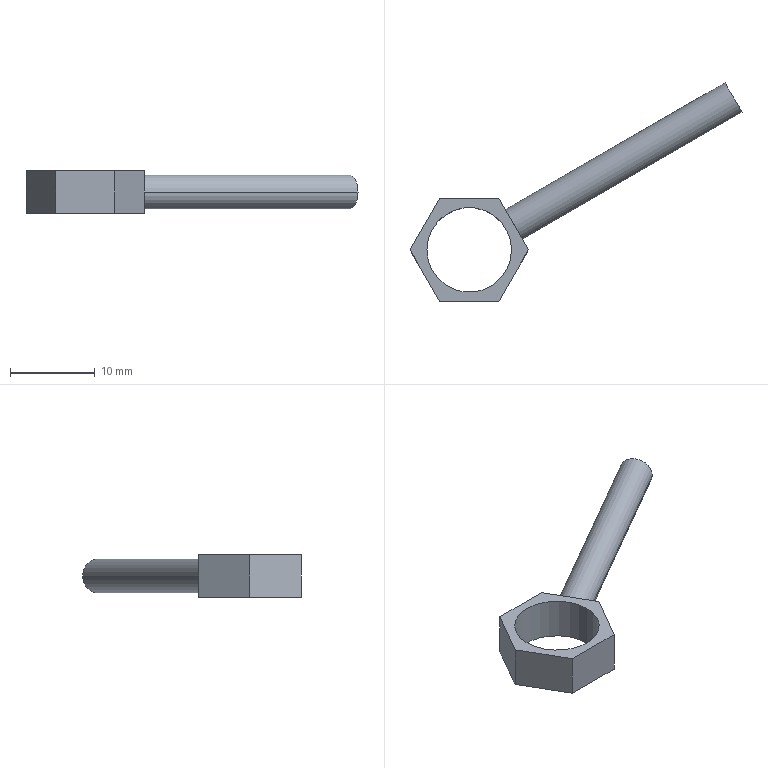Part | SolidWorks | features Extrusion 1, ICE 1 | 1 solid | 13 faces | box 39.231 x 25.825 x 5 mm | volume 620.821 mm3 | plane 9 | cylinder 4 | commonest cylinder face diameters 4 x2 10 x2
STEP:
#1=CARTESIAN_POINT('',(30.231,19.763,2.5));
#2=VERTEX_POINT('',#1);
#3=CARTESIAN_POINT('',(32.231,16.299,2.5));
#4=VERTEX_POINT('',#3);
#5=CARTESIAN_POINT('',(31.231,18.031,2.5));
#6=DIRECTION('',(0.866,0.5,0.));
#7=DIRECTION('',(-0.5,0.866,0.));
#8=AXIS2_PLACEMENT_3D('',#5,#6,#7);
#9=CIRCLE('',#8,2.);
#10=EDGE_CURVE('',#2,#4,#9,.T.);
#11=ORIENTED_EDGE('',*,*,#10,.F.);
#12=CARTESIAN_POINT('',(4.25,4.763,2.5));
#13=VERTEX_POINT('',#12);
#14=CARTESIAN_POINT('',(30.231,19.763,2.5));
#15=DIRECTION('',(-0.866,-0.5,0.));
#16=VECTOR('',#15,1000.);
#17=LINE('',#14,#16);
#18=EDGE_CURVE('',#2,#13,#17,.T.);
#19=ORIENTED_EDGE('',*,*,#18,.T.);
#20=CARTESIAN_POINT('',(6.25,1.299,2.5));
#21=VERTEX_POINT('',#20);
#22=CARTESIAN_POINT('',(5.25,3.031,2.5));
#23=DIRECTION('',(0.866,0.5,0.));
#24=DIRECTION('',(-0.5,0.866,0.));
#25=AXIS2_PLACEMENT_3D('',#22,#23,#24);
#26=CIRCLE('',#25,2.);
#27=EDGE_CURVE('',#13,#21,#26,.T.);
#28=ORIENTED_EDGE('',*,*,#27,.T.);
#29=CARTESIAN_POINT('',(32.231,16.299,2.5));
#30=DIRECTION('',(-0.866,-0.5,0.));
#31=VECTOR('',#30,1000.);
#32=LINE('',#29,#31);
#33=EDGE_CURVE('',#4,#21,#32,.T.);
#34=ORIENTED_EDGE('',*,*,#33,.F.);
#35=EDGE_LOOP('',(#11,#19,#28,#34));
#36=FACE_OUTER_BOUND('',#35,.T.);
#37=CARTESIAN_POINT('',(31.231,18.031,2.5));
#38=DIRECTION('',(-0.866,-0.5,0.));
#39=DIRECTION('',(0.5,-0.866,0.));
#40=AXIS2_PLACEMENT_3D('',#37,#38,#39);
#41=CYLINDRICAL_SURFACE('',#40,2.);
#42=ADVANCED_FACE('',(#36),#41,.T.);
#43=CARTESIAN_POINT('',(-5.,0.,5.));
#44=VERTEX_POINT('',#43);
#45=CARTESIAN_POINT('',(5.,0.,5.));
#46=VERTEX_POINT('',#45);
#47=CARTESIAN_POINT('',(0.,0.,5.));
#48=DIRECTION('',(0.,0.,1.));
#49=DIRECTION('',(1.,0.,0.));
#50=AXIS2_PLACEMENT_3D('',#47,#48,#49);
#51=CIRCLE('',#50,5.);
#52=EDGE_CURVE('',#44,#46,#51,.T.);
#53=ORIENTED_EDGE('',*,*,#52,.T.);
#54=CARTESIAN_POINT('',(5.,0.,0.));
#55=VERTEX_POINT('',#54);
#56=CARTESIAN_POINT('',(5.,0.,5.));
#57=DIRECTION('',(0.,0.,-1.));
#58=VECTOR('',#57,1000.);
#59=LINE('',#56,#58);
#60=EDGE_CURVE('',#46,#55,#59,.T.);
#61=ORIENTED_EDGE('',*,*,#60,.T.);
#62=CARTESIAN_POINT('',(-5.,0.,0.));
#63=VERTEX_POINT('',#62);
#64=CARTESIAN_POINT('',(0.,0.,0.));
#65=DIRECTION('',(0.,0.,1.));
#66=DIRECTION('',(1.,0.,0.));
#67=AXIS2_PLACEMENT_3D('',#64,#65,#66);
#68=CIRCLE('',#67,5.);
#69=EDGE_CURVE('',#63,#55,#68,.T.);
#70=ORIENTED_EDGE('',*,*,#69,.F.);
#71=CARTESIAN_POINT('',(-5.,0.,5.));
#72=DIRECTION('',(0.,0.,-1.));
#73=VECTOR('',#72,1000.);
#74=LINE('',#71,#73);
#75=EDGE_CURVE('',#44,#63,#74,.T.);
#76=ORIENTED_EDGE('',*,*,#75,.F.);
#77=EDGE_LOOP('',(#53,#61,#70,#76));
#78=FACE_OUTER_BOUND('',#77,.T.);
#79=CARTESIAN_POINT('',(0.,0.,5.));
#80=DIRECTION('',(0.,0.,-1.));
#81=DIRECTION('',(-1.,0.,0.));
#82=AXIS2_PLACEMENT_3D('',#79,#80,#81);
#83=CYLINDRICAL_SURFACE('',#82,5.);
#84=ADVANCED_FACE('',(#78),#83,.F.);
#85=CARTESIAN_POINT('',(3.5,6.062,5.));
#86=VERTEX_POINT('',#85);
#87=CARTESIAN_POINT('',(-3.5,6.062,5.));
#88=VERTEX_POINT('',#87);
#89=CARTESIAN_POINT('',(3.5,6.062,5.));
#90=DIRECTION('',(-1.,0.,0.));
#91=VECTOR('',#90,1000.);
#92=LINE('',#89,#91);
#93=EDGE_CURVE('',#86,#88,#92,.T.);
#94=ORIENTED_EDGE('',*,*,#93,.T.);
#95=CARTESIAN_POINT('',(-7.,0.,5.));
#96=VERTEX_POINT('',#95);
#97=CARTESIAN_POINT('',(-3.5,6.062,5.));
#98=DIRECTION('',(-0.5,-0.866,0.));
#99=VECTOR('',#98,1000.);
#100=LINE('',#97,#99);
#101=EDGE_CURVE('',#88,#96,#100,.T.);
#102=ORIENTED_EDGE('',*,*,#101,.T.);
#103=CARTESIAN_POINT('',(-3.5,-6.062,5.));
#104=VERTEX_POINT('',#103);
#105=CARTESIAN_POINT('',(-7.,0.,5.));
#106=DIRECTION('',(0.5,-0.866,0.));
#107=VECTOR('',#106,1000.);
#108=LINE('',#105,#107);
#109=EDGE_CURVE('',#96,#104,#108,.T.);
#110=ORIENTED_EDGE('',*,*,#109,.T.);
#111=CARTESIAN_POINT('',(3.5,-6.062,5.));
#112=VERTEX_POINT('',#111);
#113=CARTESIAN_POINT('',(-3.5,-6.062,5.));
#114=DIRECTION('',(1.,0.,0.));
#115=VECTOR('',#114,1000.);
#116=LINE('',#113,#115);
#117=EDGE_CURVE('',#104,#112,#116,.T.);
#118=ORIENTED_EDGE('',*,*,#117,.T.);
#119=CARTESIAN_POINT('',(7.,0.,5.));
#120=VERTEX_POINT('',#119);
#121=CARTESIAN_POINT('',(3.5,-6.062,5.));
#122=DIRECTION('',(0.5,0.866,0.));
#123=VECTOR('',#122,1000.);
#124=LINE('',#121,#123);
#125=EDGE_CURVE('',#112,#120,#124,.T.);
#126=ORIENTED_EDGE('',*,*,#125,.T.);
#127=CARTESIAN_POINT('',(7.,0.,5.));
#128=DIRECTION('',(-0.5,0.866,0.));
#129=VECTOR('',#128,1000.);
#130=LINE('',#127,#129);
#131=EDGE_CURVE('',#120,#86,#130,.T.);
#132=ORIENTED_EDGE('',*,*,#131,.T.);
#133=EDGE_LOOP('',(#94,#102,#110,#118,#126,#132));
#134=FACE_OUTER_BOUND('',#133,.T.);
#135=ORIENTED_EDGE('',*,*,#52,.F.);
#136=CARTESIAN_POINT('',(0.,0.,5.));
#137=DIRECTION('',(0.,0.,1.));
#138=DIRECTION('',(1.,0.,0.));
#139=AXIS2_PLACEMENT_3D('',#136,#137,#138);
#140=CIRCLE('',#139,5.);
#141=EDGE_CURVE('',#46,#44,#140,.T.);
#142=ORIENTED_EDGE('',*,*,#141,.F.);
#143=EDGE_LOOP('',(#135,#142));
#144=FACE_BOUND('',#143,.T.);
#145=CARTESIAN_POINT('',(0.,0.,5.));
#146=DIRECTION('',(0.,0.,1.));
#147=DIRECTION('',(1.,0.,0.));
#148=AXIS2_PLACEMENT_3D('',#145,#146,#147);
#149=PLANE('',#148);
#150=ADVANCED_FACE('',(#134,#144),#149,.T.);
#151=CARTESIAN_POINT('',(3.5,6.062,0.));
#152=VERTEX_POINT('',#151);
#153=CARTESIAN_POINT('',(-3.5,6.062,0.));
#154=VERTEX_POINT('',#153);
#155=CARTESIAN_POINT('',(3.5,6.062,0.));
#156=DIRECTION('',(-1.,0.,0.));
#157=VECTOR('',#156,1000.);
#158=LINE('',#155,#157);
#159=EDGE_CURVE('',#152,#154,#158,.T.);
#160=ORIENTED_EDGE('',*,*,#159,.F.);
#161=CARTESIAN_POINT('',(7.,0.,0.));
#162=VERTEX_POINT('',#161);
#163=CARTESIAN_POINT('',(7.,0.,0.));
#164=DIRECTION('',(-0.5,0.866,0.));
#165=VECTOR('',#164,1000.);
#166=LINE('',#163,#165);
#167=EDGE_CURVE('',#162,#152,#166,.T.);
#168=ORIENTED_EDGE('',*,*,#167,.F.);
#169=CARTESIAN_POINT('',(3.5,-6.062,0.));
#170=VERTEX_POINT('',#169);
#171=CARTESIAN_POINT('',(3.5,-6.062,0.));
#172=DIRECTION('',(0.5,0.866,0.));
#173=VECTOR('',#172,1000.);
#174=LINE('',#171,#173);
#175=EDGE_CURVE('',#170,#162,#174,.T.);
#176=ORIENTED_EDGE('',*,*,#175,.F.);
#177=CARTESIAN_POINT('',(-3.5,-6.062,0.));
#178=VERTEX_POINT('',#177);
#179=CARTESIAN_POINT('',(-3.5,-6.062,0.));
#180=DIRECTION('',(1.,0.,0.));
#181=VECTOR('',#180,1000.);
#182=LINE('',#179,#181);
#183=EDGE_CURVE('',#178,#170,#182,.T.);
#184=ORIENTED_EDGE('',*,*,#183,.F.);
#185=CARTESIAN_POINT('',(-7.,0.,0.));
#186=VERTEX_POINT('',#185);
#187=CARTESIAN_POINT('',(-7.,0.,0.));
#188=DIRECTION('',(0.5,-0.866,0.));
#189=VECTOR('',#188,1000.);
#190=LINE('',#187,#189);
#191=EDGE_CURVE('',#186,#178,#190,.T.);
#192=ORIENTED_EDGE('',*,*,#191,.F.);
#193=CARTESIAN_POINT('',(-3.5,6.062,0.));
#194=DIRECTION('',(-0.5,-0.866,0.));
#195=VECTOR('',#194,1000.);
#196=LINE('',#193,#195);
#197=EDGE_CURVE('',#154,#186,#196,.T.);
#198=ORIENTED_EDGE('',*,*,#197,.F.);
#199=EDGE_LOOP('',(#160,#168,#176,#184,#192,#198));
#200=FACE_OUTER_BOUND('',#199,.T.);
#201=ORIENTED_EDGE('',*,*,#69,.T.);
#202=CARTESIAN_POINT('',(0.,0.,0.));
#203=DIRECTION('',(0.,0.,1.));
#204=DIRECTION('',(1.,0.,0.));
#205=AXIS2_PLACEMENT_3D('',#202,#203,#204);
#206=CIRCLE('',#205,5.);
#207=EDGE_CURVE('',#55,#63,#206,.T.);
#208=ORIENTED_EDGE('',*,*,#207,.T.);
#209=EDGE_LOOP('',(#201,#208));
#210=FACE_BOUND('',#209,.T.);
#211=CARTESIAN_POINT('',(0.,0.,0.));
#212=DIRECTION('',(0.,0.,1.));
#213=DIRECTION('',(1.,0.,0.));
#214=AXIS2_PLACEMENT_3D('',#211,#212,#213);
#215=PLANE('',#214);
#216=ADVANCED_FACE('',(#200,#210),#215,.F.);
#217=ORIENTED_EDGE('',*,*,#159,.T.);
#218=CARTESIAN_POINT('',(-3.5,6.062,5.));
#219=DIRECTION('',(0.,0.,-1.));
#220=VECTOR('',#219,1000.);
#221=LINE('',#218,#220);
#222=EDGE_CURVE('',#88,#154,#221,.T.);
#223=ORIENTED_EDGE('',*,*,#222,.F.);
#224=ORIENTED_EDGE('',*,*,#93,.F.);
#225=CARTESIAN_POINT('',(3.5,6.062,5.));
#226=DIRECTION('',(0.,0.,-1.));
#227=VECTOR('',#226,1000.);
#228=LINE('',#225,#227);
#229=EDGE_CURVE('',#86,#152,#228,.T.);
#230=ORIENTED_EDGE('',*,*,#229,.T.);
#231=EDGE_LOOP('',(#217,#223,#224,#230));
#232=FACE_OUTER_BOUND('',#231,.T.);
#233=CARTESIAN_POINT('',(3.5,6.062,5.));
#234=DIRECTION('',(0.,-1.,0.));
#235=DIRECTION('',(1.,0.,0.));
#236=AXIS2_PLACEMENT_3D('',#233,#234,#235);
#237=PLANE('',#236);
#238=ADVANCED_FACE('',(#232),#237,.F.);
#239=ORIENTED_EDGE('',*,*,#197,.T.);
#240=CARTESIAN_POINT('',(-7.,0.,5.));
#241=DIRECTION('',(0.,0.,-1.));
#242=VECTOR('',#241,1000.);
#243=LINE('',#240,#242);
#244=EDGE_CURVE('',#96,#186,#243,.T.);
#245=ORIENTED_EDGE('',*,*,#244,.F.);
#246=ORIENTED_EDGE('',*,*,#101,.F.);
#247=ORIENTED_EDGE('',*,*,#222,.T.);
#248=EDGE_LOOP('',(#239,#245,#246,#247));
#249=FACE_OUTER_BOUND('',#248,.T.);
#250=CARTESIAN_POINT('',(-3.5,6.062,5.));
#251=DIRECTION('',(0.866,-0.5,0.));
#252=DIRECTION('',(0.5,0.866,0.));
#253=AXIS2_PLACEMENT_3D('',#250,#251,#252);
#254=PLANE('',#253);
#255=ADVANCED_FACE('',(#249),#254,.F.);
#256=ORIENTED_EDGE('',*,*,#191,.T.);
#257=CARTESIAN_POINT('',(-3.5,-6.062,5.));
#258=DIRECTION('',(0.,0.,-1.));
#259=VECTOR('',#258,1000.);
#260=LINE('',#257,#259);
#261=EDGE_CURVE('',#104,#178,#260,.T.);
#262=ORIENTED_EDGE('',*,*,#261,.F.);
#263=ORIENTED_EDGE('',*,*,#109,.F.);
#264=ORIENTED_EDGE('',*,*,#244,.T.);
#265=EDGE_LOOP('',(#256,#262,#263,#264));
#266=FACE_OUTER_BOUND('',#265,.T.);
#267=CARTESIAN_POINT('',(-7.,0.,5.));
#268=DIRECTION('',(0.866,0.5,0.));
#269=DIRECTION('',(-0.5,0.866,0.));
#270=AXIS2_PLACEMENT_3D('',#267,#268,#269);
#271=PLANE('',#270);
#272=ADVANCED_FACE('',(#266),#271,.F.);
#273=ORIENTED_EDGE('',*,*,#183,.T.);
#274=CARTESIAN_POINT('',(3.5,-6.062,5.));
#275=DIRECTION('',(0.,0.,-1.));
#276=VECTOR('',#275,1000.);
#277=LINE('',#274,#276);
#278=EDGE_CURVE('',#112,#170,#277,.T.);
#279=ORIENTED_EDGE('',*,*,#278,.F.);
#280=ORIENTED_EDGE('',*,*,#117,.F.);
#281=ORIENTED_EDGE('',*,*,#261,.T.);
#282=EDGE_LOOP('',(#273,#279,#280,#281));
#283=FACE_OUTER_BOUND('',#282,.T.);
#284=CARTESIAN_POINT('',(-3.5,-6.062,5.));
#285=DIRECTION('',(0.,1.,0.));
#286=DIRECTION('',(0.,0.,1.));
#287=AXIS2_PLACEMENT_3D('',#284,#285,#286);
#288=PLANE('',#287);
#289=ADVANCED_FACE('',(#283),#288,.F.);
#290=ORIENTED_EDGE('',*,*,#175,.T.);
#291=CARTESIAN_POINT('',(7.,0.,5.));
#292=DIRECTION('',(0.,0.,-1.));
#293=VECTOR('',#292,1000.);
#294=LINE('',#291,#293);
#295=EDGE_CURVE('',#120,#162,#294,.T.);
#296=ORIENTED_EDGE('',*,*,#295,.F.);
#297=ORIENTED_EDGE('',*,*,#125,.F.);
#298=ORIENTED_EDGE('',*,*,#278,.T.);
#299=EDGE_LOOP('',(#290,#296,#297,#298));
#300=FACE_OUTER_BOUND('',#299,.T.);
#301=CARTESIAN_POINT('',(3.5,-6.062,5.));
#302=DIRECTION('',(-0.866,0.5,0.));
#303=DIRECTION('',(-0.5,-0.866,0.));
#304=AXIS2_PLACEMENT_3D('',#301,#302,#303);
#305=PLANE('',#304);
#306=ADVANCED_FACE('',(#300),#305,.F.);
#307=CARTESIAN_POINT('',(5.25,3.031,2.5));
#308=DIRECTION('',(0.866,0.5,0.));
#309=DIRECTION('',(-0.5,0.866,0.));
#310=AXIS2_PLACEMENT_3D('',#307,#308,#309);
#311=CIRCLE('',#310,2.);
#312=EDGE_CURVE('',#21,#13,#311,.T.);
#313=ORIENTED_EDGE('',*,*,#312,.F.);
#314=ORIENTED_EDGE('',*,*,#27,.F.);
#315=EDGE_LOOP('',(#313,#314));
#316=FACE_BOUND('',#315,.T.);
#317=ORIENTED_EDGE('',*,*,#167,.T.);
#318=ORIENTED_EDGE('',*,*,#229,.F.);
#319=ORIENTED_EDGE('',*,*,#131,.F.);
#320=ORIENTED_EDGE('',*,*,#295,.T.);
#321=EDGE_LOOP('',(#317,#318,#319,#320));
#322=FACE_OUTER_BOUND('',#321,.T.);
#323=CARTESIAN_POINT('',(7.,0.,5.));
#324=DIRECTION('',(-0.866,-0.5,0.));
#325=DIRECTION('',(0.5,-0.866,0.));
#326=AXIS2_PLACEMENT_3D('',#323,#324,#325);
#327=PLANE('',#326);
#328=ADVANCED_FACE('',(#316,#322),#327,.F.);
#329=ORIENTED_EDGE('',*,*,#60,.F.);
#330=ORIENTED_EDGE('',*,*,#141,.T.);
#331=ORIENTED_EDGE('',*,*,#75,.T.);
#332=ORIENTED_EDGE('',*,*,#207,.F.);
#333=EDGE_LOOP('',(#329,#330,#331,#332));
#334=FACE_OUTER_BOUND('',#333,.T.);
#335=CARTESIAN_POINT('',(0.,0.,5.));
#336=DIRECTION('',(0.,0.,-1.));
#337=DIRECTION('',(-1.,0.,0.));
#338=AXIS2_PLACEMENT_3D('',#335,#336,#337);
#339=CYLINDRICAL_SURFACE('',#338,5.);
#340=ADVANCED_FACE('',(#334),#339,.F.);
#341=ORIENTED_EDGE('',*,*,#18,.F.);
#342=CARTESIAN_POINT('',(31.231,18.031,2.5));
#343=DIRECTION('',(0.866,0.5,0.));
#344=DIRECTION('',(-0.5,0.866,0.));
#345=AXIS2_PLACEMENT_3D('',#342,#343,#344);
#346=CIRCLE('',#345,2.);
#347=EDGE_CURVE('',#4,#2,#346,.T.);
#348=ORIENTED_EDGE('',*,*,#347,.F.);
#349=ORIENTED_EDGE('',*,*,#33,.T.);
#350=ORIENTED_EDGE('',*,*,#312,.T.);
#351=EDGE_LOOP('',(#341,#348,#349,#350));
#352=FACE_OUTER_BOUND('',#351,.T.);
#353=CARTESIAN_POINT('',(31.231,18.031,2.5));
#354=DIRECTION('',(-0.866,-0.5,0.));
#355=DIRECTION('',(0.5,-0.866,0.));
#356=AXIS2_PLACEMENT_3D('',#353,#354,#355);
#357=CYLINDRICAL_SURFACE('',#356,2.);
#358=ADVANCED_FACE('',(#352),#357,.T.);
#359=ORIENTED_EDGE('',*,*,#347,.T.);
#360=ORIENTED_EDGE('',*,*,#10,.T.);
#361=EDGE_LOOP('',(#359,#360));
#362=FACE_OUTER_BOUND('',#361,.T.);
#363=CARTESIAN_POINT('',(31.231,18.031,2.5));
#364=DIRECTION('',(0.866,0.5,0.));
#365=DIRECTION('',(-0.5,0.866,0.));
#366=AXIS2_PLACEMENT_3D('',#363,#364,#365);
#367=PLANE('',#366);
#368=ADVANCED_FACE('',(#362),#367,.T.);
#369=CLOSED_SHELL('',(#42,#84,#150,#216,#238,#255,#272,#289,#306,#328,#340,#358,#368));
#370=MANIFOLD_SOLID_BREP('',#369);
#371=CARTESIAN_POINT('',(0.,0.,0.));
#372=DIRECTION('',(0.,0.,1.));
#373=DIRECTION('',(1.,0.,0.));
#374=AXIS2_PLACEMENT_3D('',#371,#372,#373);
#375=(LENGTH_UNIT()NAMED_UNIT(*)SI_UNIT(.MILLI.,.METRE.));
#376=UNCERTAINTY_MEASURE_WITH_UNIT(LENGTH_MEASURE(0.00001),#375,'','');
#377=(NAMED_UNIT(*)PLANE_ANGLE_UNIT()SI_UNIT($,.RADIAN.));
#378=(NAMED_UNIT(*)SI_UNIT($,.STERADIAN.)SOLID_ANGLE_UNIT());
#379=(GEOMETRIC_REPRESENTATION_CONTEXT(3)GLOBAL_UNCERTAINTY_ASSIGNED_CONTEXT((#376))GLOBAL_UNIT_ASSIGNED_CONTEXT((#375,#377,#378))REPRESENTATION_CONTEXT('',''));
#380=ADVANCED_BREP_SHAPE_REPRESENTATION('',(#370,#374),#379);